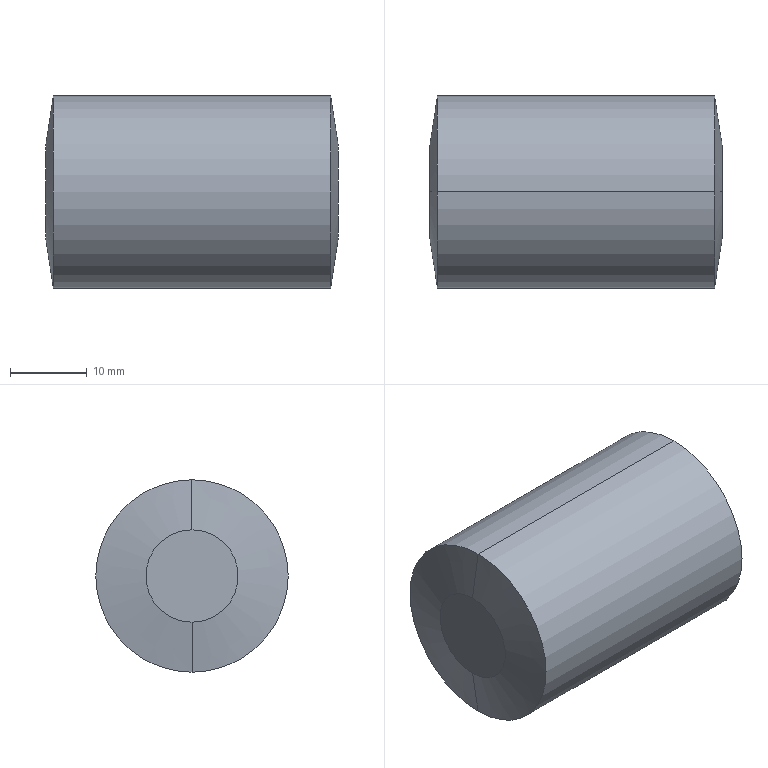Part | STEP file | SceondCKH75bearing | 1 solid | 8 faces | box 38 x 25 x 25 mm | volume 18231 mm3 | cone 4 | cylinder 2 | plane 2 | commonest cylinder face diameters 25 x2
STEP:
#1=CARTESIAN_POINT('',(19.,0.,6.));
#2=VERTEX_POINT('',#1);
#3=CARTESIAN_POINT('',(19.,0.,-6.));
#4=VERTEX_POINT('',#3);
#5=CARTESIAN_POINT('',(19.,0.,0.));
#6=DIRECTION('',(-1.,0.,0.));
#7=DIRECTION('',(0.,0.,1.));
#8=AXIS2_PLACEMENT_3D('',#5,#6,#7);
#9=CIRCLE('',#8,6.);
#10=EDGE_CURVE('',#2,#4,#9,.T.);
#11=ORIENTED_EDGE('',*,*,#10,.T.);
#12=CARTESIAN_POINT('',(18.,0.,-12.5));
#13=VERTEX_POINT('',#12);
#14=CARTESIAN_POINT('',(19.,0.,-6.));
#15=DIRECTION('',(-0.1521,0.,-0.9884));
#16=VECTOR('',#15,1000.);
#17=LINE('',#14,#16);
#18=EDGE_CURVE('',#4,#13,#17,.T.);
#19=ORIENTED_EDGE('',*,*,#18,.T.);
#20=CARTESIAN_POINT('',(18.,0.,12.5));
#21=VERTEX_POINT('',#20);
#22=CARTESIAN_POINT('',(18.,0.,0.));
#23=DIRECTION('',(-1.,0.,0.));
#24=DIRECTION('',(0.,0.,1.));
#25=AXIS2_PLACEMENT_3D('',#22,#23,#24);
#26=CIRCLE('',#25,12.5);
#27=EDGE_CURVE('',#21,#13,#26,.T.);
#28=ORIENTED_EDGE('',*,*,#27,.F.);
#29=CARTESIAN_POINT('',(19.,0.,6.));
#30=DIRECTION('',(-0.1521,0.,0.9884));
#31=VECTOR('',#30,1000.);
#32=LINE('',#29,#31);
#33=EDGE_CURVE('',#2,#21,#32,.T.);
#34=ORIENTED_EDGE('',*,*,#33,.F.);
#35=EDGE_LOOP('',(#11,#19,#28,#34));
#36=FACE_OUTER_BOUND('',#35,.T.);
#37=CARTESIAN_POINT('',(19.,0.,0.));
#38=DIRECTION('',(-1.,0.,0.));
#39=DIRECTION('',(0.,0.,1.));
#40=AXIS2_PLACEMENT_3D('',#37,#38,#39);
#41=CONICAL_SURFACE('',#40,6.,1.418);
#42=ADVANCED_FACE('',(#36),#41,.T.);
#43=ORIENTED_EDGE('',*,*,#27,.T.);
#44=CARTESIAN_POINT('',(-18.,0.,-12.5));
#45=VERTEX_POINT('',#44);
#46=CARTESIAN_POINT('',(19.,0.,-12.5));
#47=DIRECTION('',(-1.,0.,0.));
#48=VECTOR('',#47,1000.);
#49=LINE('',#46,#48);
#50=EDGE_CURVE('',#13,#45,#49,.T.);
#51=ORIENTED_EDGE('',*,*,#50,.T.);
#52=CARTESIAN_POINT('',(-18.,0.,12.5));
#53=VERTEX_POINT('',#52);
#54=CARTESIAN_POINT('',(-18.,0.,0.));
#55=DIRECTION('',(-1.,0.,0.));
#56=DIRECTION('',(0.,0.,1.));
#57=AXIS2_PLACEMENT_3D('',#54,#55,#56);
#58=CIRCLE('',#57,12.5);
#59=EDGE_CURVE('',#53,#45,#58,.T.);
#60=ORIENTED_EDGE('',*,*,#59,.F.);
#61=CARTESIAN_POINT('',(19.,0.,12.5));
#62=DIRECTION('',(-1.,0.,0.));
#63=VECTOR('',#62,1000.);
#64=LINE('',#61,#63);
#65=EDGE_CURVE('',#21,#53,#64,.T.);
#66=ORIENTED_EDGE('',*,*,#65,.F.);
#67=EDGE_LOOP('',(#43,#51,#60,#66));
#68=FACE_OUTER_BOUND('',#67,.T.);
#69=CARTESIAN_POINT('',(19.,0.,0.));
#70=DIRECTION('',(-1.,0.,0.));
#71=DIRECTION('',(0.,0.,1.));
#72=AXIS2_PLACEMENT_3D('',#69,#70,#71);
#73=CYLINDRICAL_SURFACE('',#72,12.5);
#74=ADVANCED_FACE('',(#68),#73,.T.);
#75=CARTESIAN_POINT('',(-19.,0.,6.));
#76=VERTEX_POINT('',#75);
#77=CARTESIAN_POINT('',(-19.,0.,-6.));
#78=VERTEX_POINT('',#77);
#79=CARTESIAN_POINT('',(-19.,0.,0.));
#80=DIRECTION('',(-1.,0.,0.));
#81=DIRECTION('',(0.,0.,1.));
#82=AXIS2_PLACEMENT_3D('',#79,#80,#81);
#83=CIRCLE('',#82,6.);
#84=EDGE_CURVE('',#76,#78,#83,.T.);
#85=ORIENTED_EDGE('',*,*,#84,.F.);
#86=CARTESIAN_POINT('',(-18.,0.,12.5));
#87=DIRECTION('',(0.1521,0.,0.9884));
#88=VECTOR('',#87,1000.);
#89=LINE('',#86,#88);
#90=EDGE_CURVE('',#76,#53,#89,.T.);
#91=ORIENTED_EDGE('',*,*,#90,.T.);
#92=ORIENTED_EDGE('',*,*,#59,.T.);
#93=CARTESIAN_POINT('',(-18.,0.,-12.5));
#94=DIRECTION('',(0.1521,0.,-0.9884));
#95=VECTOR('',#94,1000.);
#96=LINE('',#93,#95);
#97=EDGE_CURVE('',#78,#45,#96,.T.);
#98=ORIENTED_EDGE('',*,*,#97,.F.);
#99=EDGE_LOOP('',(#85,#91,#92,#98));
#100=FACE_OUTER_BOUND('',#99,.T.);
#101=CARTESIAN_POINT('',(-18.,0.,0.));
#102=DIRECTION('',(1.,0.,0.));
#103=DIRECTION('',(0.,0.,-1.));
#104=AXIS2_PLACEMENT_3D('',#101,#102,#103);
#105=CONICAL_SURFACE('',#104,12.5,1.418);
#106=ADVANCED_FACE('',(#100),#105,.T.);
#107=CARTESIAN_POINT('',(-19.,0.,0.));
#108=DIRECTION('',(-1.,0.,0.));
#109=DIRECTION('',(0.,0.,1.));
#110=AXIS2_PLACEMENT_3D('',#107,#108,#109);
#111=CIRCLE('',#110,6.);
#112=EDGE_CURVE('',#78,#76,#111,.T.);
#113=ORIENTED_EDGE('',*,*,#112,.T.);
#114=ORIENTED_EDGE('',*,*,#84,.T.);
#115=EDGE_LOOP('',(#113,#114));
#116=FACE_OUTER_BOUND('',#115,.T.);
#117=CARTESIAN_POINT('',(-19.,0.,0.));
#118=DIRECTION('',(1.,0.,0.));
#119=DIRECTION('',(0.,0.,-1.));
#120=AXIS2_PLACEMENT_3D('',#117,#118,#119);
#121=PLANE('',#120);
#122=ADVANCED_FACE('',(#116),#121,.F.);
#123=ORIENTED_EDGE('',*,*,#90,.F.);
#124=ORIENTED_EDGE('',*,*,#112,.F.);
#125=ORIENTED_EDGE('',*,*,#97,.T.);
#126=CARTESIAN_POINT('',(-18.,0.,0.));
#127=DIRECTION('',(-1.,0.,0.));
#128=DIRECTION('',(0.,0.,1.));
#129=AXIS2_PLACEMENT_3D('',#126,#127,#128);
#130=CIRCLE('',#129,12.5);
#131=EDGE_CURVE('',#45,#53,#130,.T.);
#132=ORIENTED_EDGE('',*,*,#131,.T.);
#133=EDGE_LOOP('',(#123,#124,#125,#132));
#134=FACE_OUTER_BOUND('',#133,.T.);
#135=CARTESIAN_POINT('',(-18.,0.,0.));
#136=DIRECTION('',(1.,0.,0.));
#137=DIRECTION('',(0.,0.,-1.));
#138=AXIS2_PLACEMENT_3D('',#135,#136,#137);
#139=CONICAL_SURFACE('',#138,12.5,1.418);
#140=ADVANCED_FACE('',(#134),#139,.T.);
#141=ORIENTED_EDGE('',*,*,#50,.F.);
#142=CARTESIAN_POINT('',(18.,0.,0.));
#143=DIRECTION('',(-1.,0.,0.));
#144=DIRECTION('',(0.,0.,1.));
#145=AXIS2_PLACEMENT_3D('',#142,#143,#144);
#146=CIRCLE('',#145,12.5);
#147=EDGE_CURVE('',#13,#21,#146,.T.);
#148=ORIENTED_EDGE('',*,*,#147,.T.);
#149=ORIENTED_EDGE('',*,*,#65,.T.);
#150=ORIENTED_EDGE('',*,*,#131,.F.);
#151=EDGE_LOOP('',(#141,#148,#149,#150));
#152=FACE_OUTER_BOUND('',#151,.T.);
#153=CARTESIAN_POINT('',(19.,0.,0.));
#154=DIRECTION('',(-1.,0.,0.));
#155=DIRECTION('',(0.,0.,1.));
#156=AXIS2_PLACEMENT_3D('',#153,#154,#155);
#157=CYLINDRICAL_SURFACE('',#156,12.5);
#158=ADVANCED_FACE('',(#152),#157,.T.);
#159=ORIENTED_EDGE('',*,*,#18,.F.);
#160=CARTESIAN_POINT('',(19.,0.,0.));
#161=DIRECTION('',(-1.,0.,0.));
#162=DIRECTION('',(0.,0.,1.));
#163=AXIS2_PLACEMENT_3D('',#160,#161,#162);
#164=CIRCLE('',#163,6.);
#165=EDGE_CURVE('',#4,#2,#164,.T.);
#166=ORIENTED_EDGE('',*,*,#165,.T.);
#167=ORIENTED_EDGE('',*,*,#33,.T.);
#168=ORIENTED_EDGE('',*,*,#147,.F.);
#169=EDGE_LOOP('',(#159,#166,#167,#168));
#170=FACE_OUTER_BOUND('',#169,.T.);
#171=CARTESIAN_POINT('',(19.,0.,0.));
#172=DIRECTION('',(-1.,0.,0.));
#173=DIRECTION('',(0.,0.,1.));
#174=AXIS2_PLACEMENT_3D('',#171,#172,#173);
#175=CONICAL_SURFACE('',#174,6.,1.418);
#176=ADVANCED_FACE('',(#170),#175,.T.);
#177=ORIENTED_EDGE('',*,*,#10,.F.);
#178=ORIENTED_EDGE('',*,*,#165,.F.);
#179=EDGE_LOOP('',(#177,#178));
#180=FACE_OUTER_BOUND('',#179,.T.);
#181=CARTESIAN_POINT('',(19.,6.,0.));
#182=DIRECTION('',(-1.,0.,0.));
#183=DIRECTION('',(0.,0.,1.));
#184=AXIS2_PLACEMENT_3D('',#181,#182,#183);
#185=PLANE('',#184);
#186=ADVANCED_FACE('',(#180),#185,.F.);
#187=CLOSED_SHELL('',(#42,#74,#106,#122,#140,#158,#176,#186));
#188=MANIFOLD_SOLID_BREP('',#187);
#189=CARTESIAN_POINT('',(0.,0.,0.));
#190=DIRECTION('',(0.,0.,1.));
#191=DIRECTION('',(1.,0.,0.));
#192=AXIS2_PLACEMENT_3D('',#189,#190,#191);
#193=(LENGTH_UNIT()NAMED_UNIT(*)SI_UNIT(.MILLI.,.METRE.));
#194=UNCERTAINTY_MEASURE_WITH_UNIT(LENGTH_MEASURE(0.00001),#193,'','');
#195=(NAMED_UNIT(*)PLANE_ANGLE_UNIT()SI_UNIT($,.RADIAN.));
#196=(NAMED_UNIT(*)SI_UNIT($,.STERADIAN.)SOLID_ANGLE_UNIT());
#197=(GEOMETRIC_REPRESENTATION_CONTEXT(3)GLOBAL_UNCERTAINTY_ASSIGNED_CONTEXT((#194))GLOBAL_UNIT_ASSIGNED_CONTEXT((#193,#195,#196))REPRESENTATION_CONTEXT('',''));
#198=ADVANCED_BREP_SHAPE_REPRESENTATION('',(#188,#192),#197);